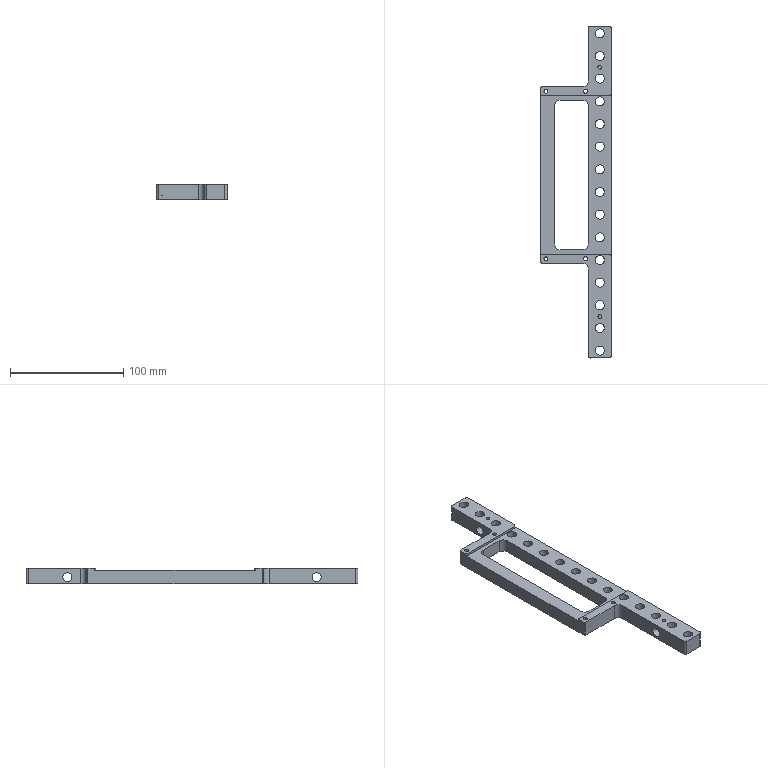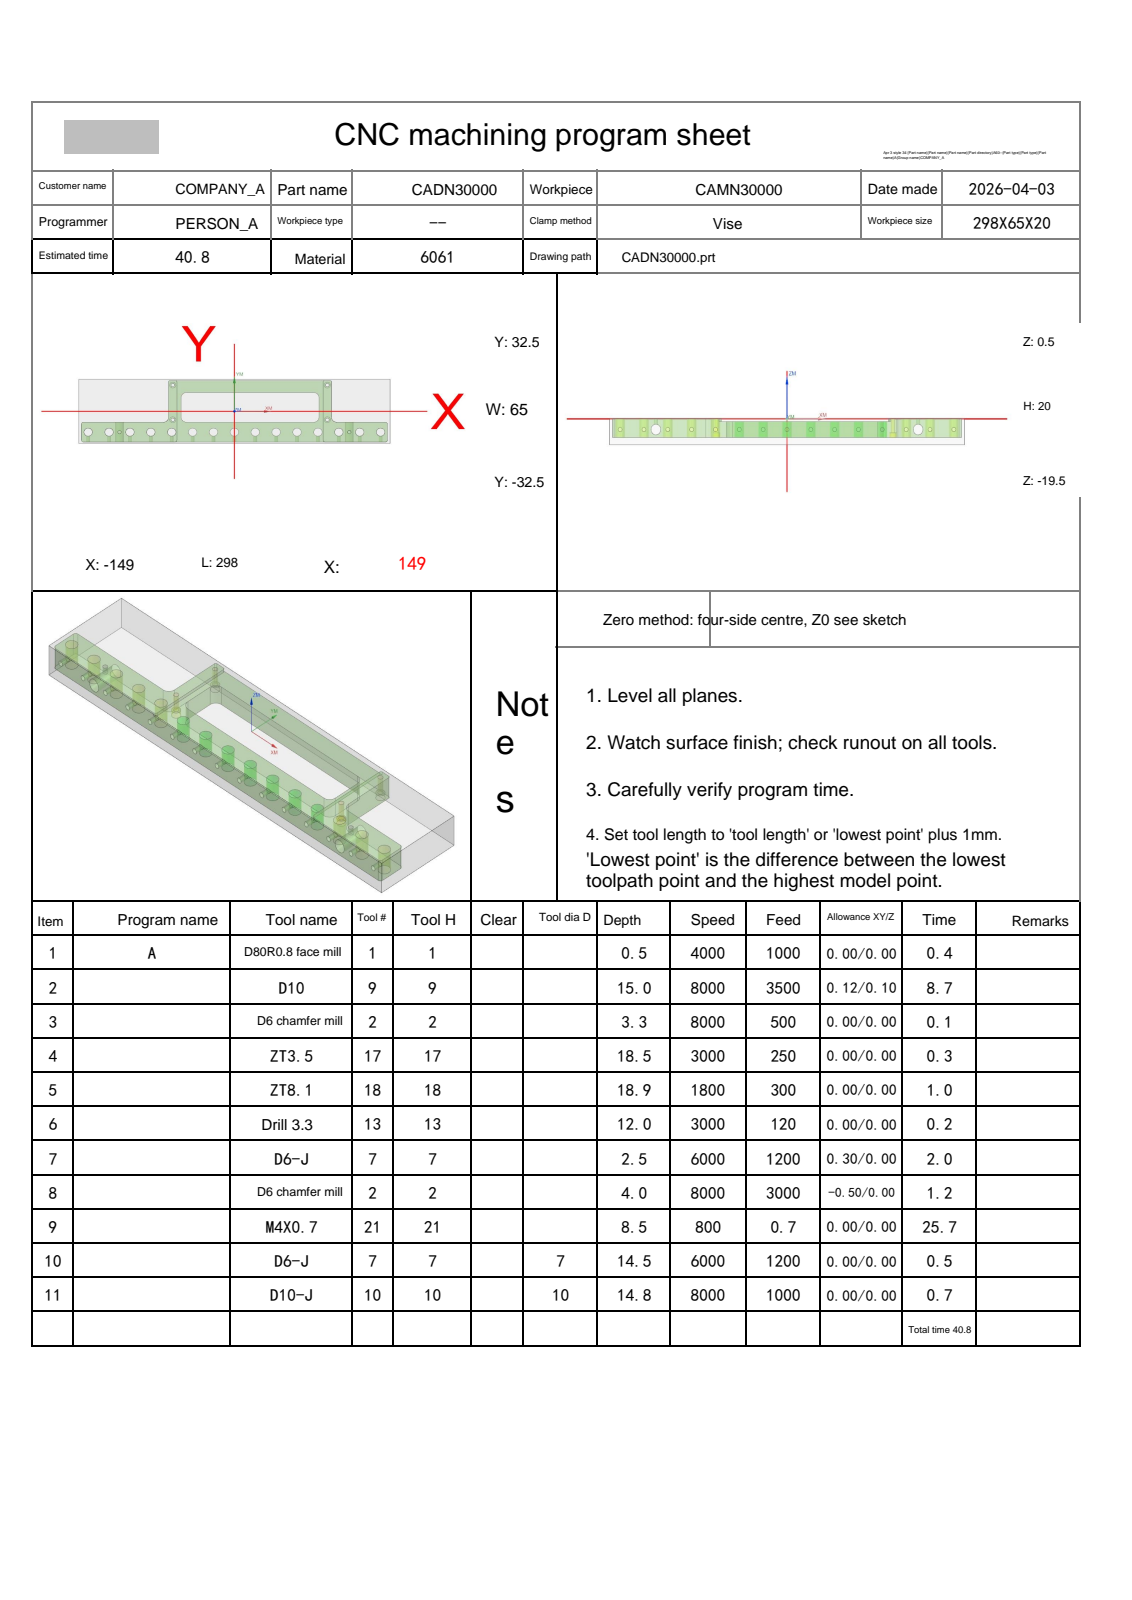NC program | NX | posted by the shop | part box 62 x 293 x 14 mm
Lines 5279 to 5964 of 5964:
N3 T02 M06
(D6 chamfer mill  D=6. R=0. H=02 ce=0.00 di=0.10)
G00 G90 G54 X-140. Y-21. M03 S8000
G43 H02 Z20.
M08
G98 G81 X-140. Y-21. Z-.8 R1. F500.
X-120.
X-110.
X-100.
X-80.
X-60.
X-59. Y-8.5
Y26.5
X-40. Y-21. Z-2.8 R-1.
X-20.
X0.0
X20.
X40.
X60.
X80.
X89. Y-8.5 Z-.8 R1.
Y26.5
X100. Y-21.
X110.
X120.
X140.
G80
G00 Z20.
G91 G28 Z0.0
M05
M09
G91 G28 Z0.0
M01
N4 T17 M06
(ZT3.5 D=3.5 DR_a=118 H=17)
G00 G90 G54 X-59. Y26.5 M03 S3000
G43 H17 Z20.
M08
G98 G83 X-59. Y26.5 Z-18. R1. F250. Q3.
Y-8.5
X89.
Y26.5
G80
G00 Z20.
G91 G28 Z0.0
M05
M09
G91 G28 Z0.0
M01
N5 T18 M06
(ZT8.1 D=8.1 DR_a=118 H=18)
G00 G90 G54 X140. Y-21. M03 S1800
G43 H18 Z20.
M08
G98 G83 X140. Y-21. Z-18.433 R1. F300. Q3.
X120.
X100.
G98 G83 X80. Y-21. Z-18.433 R-1. Q3.
X60.
X40.
X20.
X0.0
X-20.
X-40.
G98 G83 X-60. Y-21. Z-18.433 R1. Q3.
X-80.
X-100.
X-120.
X-140.
G80
G00 Z20.
G91 G28 Z0.0
M05
M09
G91 G28 Z0.0
M01
N6 T13 M06
(drill 3.3 D=3.3 DR_a=118 H=13)
G00 G90 G54 X110. Y-21. M03 S3000
G43 H13 Z20.
M08
G98 G83 X110. Y-21. Z-11.5 R1. F120. Q2.
X-110.
G80
G00 Z20.
G91 G28 Z0.0
M05
M09
G91 G28 Z0.0
M01
N7 T07 M06
(D6-J  D=6. R=0. H=07 ce=0.30 di=0.00)
G00 G90 G54 X14.056 Y-37. M03 S6000
G43 H07 Z20.
M08
Z-1.5
G01 Z-2. F1200.
X14.253 Y-31.6
G03 X14.3 Y-29. I-71.253 J2.6
G01 Y30.
G03 X14.282 Y31.6 I-70.3 J0.0
G01 X14.159 Y37.
Z-1.5
G00 Z20.
X15.841
Z-1.5
G01 Z-2.
X15.718 Y31.6
G03 X15.7 Y30. I70.282 J-1.6
G01 Y-29.
G03 X15.747 Y-31.6 I71.3 J0.0
G01 X15.944 Y-37.
Z-1.5
G00 Z20.
X11.045
Z-1.5
G01 Z-2.
X11.25 Y-31.6
G03 X11.3 Y-29. I-68.25 J2.6
G01 Y30.
G03 X11.281 Y31.6 I-67.3 J0.0
G01 X7.08
G02 X7.1 Y30. I-63.08 J-1.6
G01 Y-29.
G02 X7.047 Y-31.6 I-64.1 J0.0
G01 X2.844
G03 X2.9 Y-29. I-59.844 J2.6
G01 Y30.
G03 X2.878 Y31.6 I-58.9 J0.0
G01 X-1.323
G02 X-1.3 Y30. I-54.677 J-1.6
G01 Y-29.
G02 X-1.361 Y-31.6 I-55.7 J0.0
G01 X-5.566
G03 X-5.5 Y-29. I-51.434 J2.6
G01 Y30.
G03 X-5.525 Y31.6 I-50.5 J0.0
G01 X-9.728
G02 X-9.7 Y30. I-46.272 J-1.6
G01 Y-29.
G02 X-9.772 Y-31.6 I-47.3 J0.0
G01 X-13.978
G03 X-13.9 Y-29. I-43.022 J2.6
G01 Y30.
G03 X-13.93 Y31.6 I-42.1 J0.0
G01 X-18.134
G02 X-18.1 Y30. I-37.866 J-1.6
G01 Y-29.
G02 X-18.187 Y-31.6 I-38.9 J0.0
G01 X-22.398
G03 X-22.3 Y-29. I-34.602 J2.6
G01 Y30.
G03 X-22.338 Y31.6 I-33.7 J0.0
G01 X-26.543
G02 X-26.5 Y30. I-29.457 J-1.6
G01 Y-29.
G02 X-26.611 Y-31.6 I-30.5 J0.0
G01 X-30.829
G03 X-30.7 Y-29. I-26.171 J2.6
G01 Y30.
G03 X-30.751 Y31.6 I-25.3 J0.0
G01 X-34.961
G02 X-34.9 Y30. I-21.039 J-1.6
G01 Y-29.
G02 X-35.053 Y-31.6 I-22.1 J0.0
G01 X-39.29
G03 X-39.1 Y-29. I-17.71 J2.6
G01 Y30.
G03 X-39.176 Y31.6 I-16.9 J0.0
G01 X-43.401
G02 X-43.3 Y30. I-12.599 J-1.6
G01 Y-29.
G02 X-43.549 Y-31.6 I-13.7 J0.0
G01 X-47.863
G03 X-47.5 Y-29. I-9.137 J2.6
G01 Y30.
G03 X-47.652 Y31.6 I-8.5 J0.0
G01 X-52.009
G02 X-51.7 Y30. I-3.991 J-1.6
G01 Y-29.
G02 X-52.382 Y-31.6 I-5.3 J0.0
G01 X-55.515 Y-37.166
Z-1.5
G00 Z20.
X18.847 Y37.
Z-1.5
G01 Z-2.
X18.719 Y31.6
G03 X18.7 Y30. I67.281 J-1.6
G01 Y-29.
G03 X18.75 Y-31.6 I68.3 J0.0
G01 X22.953
G02 X22.9 Y-29. I64.047 J2.6
G01 Y30.
G02 X22.92 Y31.6 I63.1 J0.0
G01 X27.122
G03 X27.1 Y30. I58.878 J-1.6
G01 Y-29.
G03 X27.156 Y-31.6 I59.9 J0.0
G01 X31.361
G02 X31.3 Y-29. I55.639 J2.6
G01 Y30.
G02 X31.323 Y31.6 I54.7 J0.0
G01 X35.525
G03 X35.5 Y30. I50.475 J-1.6
G01 Y-29.
G03 X35.566 Y-31.6 I51.5 J0.0
G01 X39.772
G02 X39.7 Y-29. I47.228 J2.6
G01 Y30.
G02 X39.728 Y31.6 I46.3 J0.0
G01 X43.93
G03 X43.9 Y30. I42.07 J-1.6
G01 Y-29.
G03 X43.978 Y-31.6 I43.1 J0.0
G01 X48.187
G02 X48.1 Y-29. I38.813 J2.6
G01 Y30.
G02 X48.134 Y31.6 I37.9 J0.0
G01 X52.338
G03 X52.3 Y30. I33.662 J-1.6
G01 Y-29.
G03 X52.398 Y-31.6 I34.7 J0.0
G01 X56.611
G02 X56.5 Y-29. I30.389 J2.6
G01 Y30.
G02 X56.543 Y31.6 I29.5 J0.0
G01 X60.751
G03 X60.7 Y30. I25.249 J-1.6
G01 Y-29.
G03 X60.829 Y-31.6 I26.3 J0.0
G01 X65.053
G02 X64.9 Y-29. I21.947 J2.6
G01 Y30.
G02 X64.961 Y31.6 I21.1 J0.0
G01 X69.176
G03 X69.1 Y30. I16.824 J-1.6
G01 Y-29.
G03 X69.29 Y-31.6 I17.9 J0.0
G01 X73.549
G02 X73.3 Y-29. I13.451 J2.6
G01 Y30.
G02 X73.401 Y31.6 I12.7 J0.0
G01 X77.652
G03 X77.5 Y30. I8.348 J-1.6
G01 Y-29.
G03 X77.863 Y-31.6 I9.5 J0.0
G01 X82.382
G02 X81.7 Y-29. I4.618 J2.6
G01 Y30.
G02 X82.009 Y31.6 I4.3 J0.0
G01 X84.204 Y37.076
Z-1.5
G00 Z20.
G91 G28 Z0.0
M05
M09
G91 G28 Z0.0
M01
N8 T02 M06
(D6 chamfer mill  D=6. R=0. H=02 ce=0.00 di=0.00)
G00 G90 G54 X83.172 Y.25 M03 S8000
G43 H02 Z20.
M08
Z2.399
G01 Z-1.5 F3000.
G03 X83.472 Y.17 I.3 J.52
X83.992 Y.47 I0.0 J.6
G01 X84. Y.5
Y30.
G02 X86. Y32. I2. J0.0
G01 X92.
G02 X94. Y30. I0.0 J-2.
G01 Y-5.9
G03 X98.1 Y-10. I4.1 J0.0
G01 X144.5
G02 X147.5 Y-13. I0.0 J-3.
G01 Y-29.
G02 X144.5 Y-32. I-3. J0.0
G01 X87.
G02 X84. Y-29. I0.0 J3.
G01 Y.5
X83.992 Y.53
G03 X83.472 Y.83 I-.52 J-.3
X83.172 Y.75 I0.0 J-.6
G01 Z2.399
G00 Z20.
X-100.5 Y-32.828
Z2.399
G01 Z-1.5
G03 X-100.42 Y-32.528 I-.52 J.3
X-100.72 Y-32.008 I-.6 J0.0
G01 X-100.75 Y-32.
X-144.5
G02 X-147.5 Y-29. I0.0 J3.
G01 Y-13.
G02 X-144.5 Y-10. I3. J0.0
G01 X-68.1
G03 X-64. Y-5.9 I0.0 J4.1
G01 Y30.
G02 X-62. Y32. I2. J0.0
G01 X-56.
G02 X-54. Y30. I0.0 J-2.
G01 Y-29.
G02 X-57. Y-32. I-3. J0.0
G01 X-100.75
X-100.78 Y-32.008
G03 X-101.08 Y-32.528 I.3 J-.52
X-101. Y-32.828 I.6 J0.0
G01 Z2.399
G00 Z20.
X-52.193 Y32.828
Z2.055
G01 Z-3.5
G03 X-52.274 Y32.528 I.52 J-.3
X-51.974 Y32.008 I.6 J0.0
G01 X-51.944 Y32.
X81.944
X81.974 Y32.008
G03 X82.274 Y32.528 I-.3 J.52
X82.193 Y32.828 I-.6 J0.0
G01 Z2.055
G00 Z20.
X82.609 Y-32.828
Z2.055
G01 Z-3.5
G03 X82.689 Y-32.528 I-.52 J.3
X82.389 Y-32.008 I-.6 J0.0
G01 X82.359 Y-32.
X-52.359
X-52.389 Y-32.008
G03 X-52.689 Y-32.528 I.3 J-.52
X-52.609 Y-32.828 I.6 J0.0
G01 Z2.055
G00 Z20.
X14.75 Y-9.172
Z.399
G01 Z-3.5
G03 X14.67 Y-9.472 I.52 J-.3
X14.97 Y-9.992 I.6 J0.0
G01 X15. Y-10.
X75.9
G03 X80. Y-5.9 I0.0 J4.1
G01 Y13.9
G03 X75.9 Y18. I-4.1 J0.0
G01 X-45.9
G03 X-50. Y13.9 I0.0 J-4.1
G01 Y-5.9
G03 X-45.9 Y-10. I4.1 J0.0
G01 X15.
X15.03 Y-9.992
G03 X15.33 Y-9.472 I-.3 J.52
X15.25 Y-9.172 I-.6 J0.0
G01 Z.399
G00 Z20.
G00 G90 X110. Y-21. M03 S8000
Z20.
G98 G81 X110. Y-21. Z-2.2 R3. F500.
X-110.
G80
G00 Z20.
G00 G90 X-59. Y26.5 M03 S8000
Z20.
G98 G81 X-59. Y26.5 Z-2.05 R3. F500.
Y-8.5
X89.
Y26.5
G80
G00 Z20.
G00 G90 X-137.492 Y-20.54 M03 S8000
Z20.
Z-.5
G01 Z-1. F800.
X-137. Y-20.45
G03 X-140. Y-17.45 I-3. J0.0
X-143.55 Y-21. I0.0 J-3.55
X-140. Y-24.55 I3.55 J0.0
X-136.45 Y-21. I0.0 J3.55
X-140. Y-17.45 I-3.55 J0.0
X-143. Y-20.45 I0.0 J-3.
G01 X-142.508 Y-20.54
Z-.5
G00 Z20.
X-117.492
Z-.5
G01 Z-1.
X-117. Y-20.45
G03 X-120. Y-17.45 I-3. J0.0
X-123.55 Y-21. I0.0 J-3.55
X-120. Y-24.55 I3.55 J0.0
X-116.45 Y-21. I0.0 J3.55
X-120. Y-17.45 I-3.55 J0.0
X-123. Y-20.45 I0.0 J-3.
G01 X-122.508 Y-20.54
Z-.5
G00 Z20.
X-97.492
Z-.5
G01 Z-1.
X-97. Y-20.45
G03 X-100. Y-17.45 I-3. J0.0
X-103.55 Y-21. I0.0 J-3.55
X-100. Y-24.55 I3.55 J0.0
X-96.45 Y-21. I0.0 J3.55
X-100. Y-17.45 I-3.55 J0.0
X-103. Y-20.45 I0.0 J-3.
G01 X-102.508 Y-20.54
Z-.5
G00 Z20.
X-77.492
Z-.5
G01 Z-1.
X-77. Y-20.45
G03 X-80. Y-17.45 I-3. J0.0
X-83.55 Y-21. I0.0 J-3.55
X-80. Y-24.55 I3.55 J0.0
X-76.45 Y-21. I0.0 J3.55
X-80. Y-17.45 I-3.55 J0.0
X-83. Y-20.45 I0.0 J-3.
G01 X-82.508 Y-20.54
Z-.5
G00 Z20.
X-57.492
Z-.5
G01 Z-1.
X-57. Y-20.45
G03 X-60. Y-17.45 I-3. J0.0
X-63.55 Y-21. I0.0 J-3.55
X-60. Y-24.55 I3.55 J0.0
X-56.45 Y-21. I0.0 J3.55
X-60. Y-17.45 I-3.55 J0.0
X-63. Y-20.45 I0.0 J-3.
G01 X-62.508 Y-20.54
Z-.5
G00 Z20.
X-39.45 Y-20.982
Z-.5
G01 Z-1.
X-38.5 Y-20.95
G03 X-40. Y-19.45 I-1.5 J0.0
X-41.55 Y-21. I0.0 J-1.55
X-40. Y-22.55 I1.55 J0.0
X-38.45 Y-21. I0.0 J1.55
X-40. Y-19.45 I-1.55 J0.0
X-41.5 Y-20.95 I0.0 J-1.5
G01 X-40.55 Y-20.982
Z-.5
G00 Z20.
X-19.45
Z-.5
G01 Z-1.
X-18.5 Y-20.95
G03 X-20. Y-19.45 I-1.5 J0.0
X-21.55 Y-21. I0.0 J-1.55
X-20. Y-22.55 I1.55 J0.0
X-18.45 Y-21. I0.0 J1.55
X-20. Y-19.45 I-1.55 J0.0
X-21.5 Y-20.95 I0.0 J-1.5
G01 X-20.55 Y-20.982
Z-.5
G00 Z20.
X.55
Z-.5
G01 Z-1.
X1.5 Y-20.95
G03 X0.0 Y-19.45 I-1.5 J0.0
X-1.55 Y-21. I0.0 J-1.55
X0.0 Y-22.55 I1.55 J0.0
X1.55 Y-21. I0.0 J1.55
X0.0 Y-19.45 I-1.55 J0.0
X-1.5 Y-20.95 I0.0 J-1.5
G01 X-.55 Y-20.982
Z-.5
G00 Z20.
X20.55
Z-.5
G01 Z-1.
X21.5 Y-20.95
G03 X20. Y-19.45 I-1.5 J0.0
X18.45 Y-21. I0.0 J-1.55
X20. Y-22.55 I1.55 J0.0
X21.55 Y-21. I0.0 J1.55
X20. Y-19.45 I-1.55 J0.0
X18.5 Y-20.95 I0.0 J-1.5
G01 X19.45 Y-20.982
Z-.5
G00 Z20.
X40.55
Z-.5
G01 Z-1.
X41.5 Y-20.95
G03 X40. Y-19.45 I-1.5 J0.0
X38.45 Y-21. I0.0 J-1.55
X40. Y-22.55 I1.55 J0.0
X41.55 Y-21. I0.0 J1.55
X40. Y-19.45 I-1.55 J0.0
X38.5 Y-20.95 I0.0 J-1.5
G01 X39.45 Y-20.982
Z-.5
G00 Z20.
X60.55
Z-.5
G01 Z-1.
X61.5 Y-20.95
G03 X60. Y-19.45 I-1.5 J0.0
X58.45 Y-21. I0.0 J-1.55
X60. Y-22.55 I1.55 J0.0
X61.55 Y-21. I0.0 J1.55
X60. Y-19.45 I-1.55 J0.0
X58.5 Y-20.95 I0.0 J-1.5
G01 X59.45 Y-20.982
Z-.5
G00 Z20.
X80.55
Z-.5
G01 Z-1.
X81.5 Y-20.95
G03 X80. Y-19.45 I-1.5 J0.0
X78.45 Y-21. I0.0 J-1.55
X80. Y-22.55 I1.55 J0.0
X81.55 Y-21. I0.0 J1.55
X80. Y-19.45 I-1.55 J0.0
X78.5 Y-20.95 I0.0 J-1.5
G01 X79.45 Y-20.982
Z-.5
G00 Z20.
X102.508 Y-20.54
Z-.5
G01 Z-1.
X103. Y-20.45
G03 X100. Y-17.45 I-3. J0.0
X96.45 Y-21. I0.0 J-3.55
X100. Y-24.55 I3.55 J0.0
X103.55 Y-21. I0.0 J3.55
X100. Y-17.45 I-3.55 J0.0
X97. Y-20.45 I0.0 J-3.
G01 X97.492 Y-20.54
Z-.5
G00 Z20.
X122.508
Z-.5
G01 Z-1.
X123. Y-20.45
G03 X120. Y-17.45 I-3. J0.0
X116.45 Y-21. I0.0 J-3.55
X120. Y-24.55 I3.55 J0.0
X123.55 Y-21. I0.0 J3.55
X120. Y-17.45 I-3.55 J0.0
X117. Y-20.45 I0.0 J-3.
G01 X117.492 Y-20.54
Z-.5
G00 Z20.
X142.508
Z-.5
G01 Z-1.
X143. Y-20.45
G03 X140. Y-17.45 I-3. J0.0
X136.45 Y-21. I0.0 J-3.55
X140. Y-24.55 I3.55 J0.0
X143.55 Y-21. I0.0 J3.55
X140. Y-17.45 I-3.55 J0.0
X137. Y-20.45 I0.0 J-3.
G01 X137.492 Y-20.54
Z-.5
G00 Z20.
G91 G28 Z0.0
M05
M09
G91 G28 Z0.0
M01
N9 T21 M06
(M4X0.7 D=3.3 DR_a=180 H=21)
G00 G90 G54 X110. Y-21. M03 S800
G43 H21 Z20.
M08
G95
G98 G84 X110. Y-21. Z-8. R1. F.7 Q3.
X-110.
G80
G94
G00 Z20.
G91 G28 Z0.0
M05
M09
G91 G28 Z0.0
M01
N10 T07 M06
(D6-J  D=6. R=0. H=07 ce=0.00 di=0.01)
G00 G90 G54 X90.7 Y-35.1 M03 S6000
G43 H07 Z20.
M08
Z-1.495
G01 Z-1.995 F1200.
G41 D07
Y-35.
G03 X89.7 Y-34. I-1. J0.0
G01 X87.
G02 X82. Y-29. I0.0 J5.
G01 Y30.
G02 X86. Y34. I4. J0.0
G01 X88.7
G03 X89.7 Y35. I0.0 J1.
G01 G40 Y35.1
Z-1.495
G00 Z20.
X-59.7
Z-1.495
G01 Z-1.995
G41 D07
Y35.
G03 X-58.7 Y34. I1. J0.0
G01 X-56.
G02 X-52. Y30. I0.0 J-4.
G01 Y-29.
G02 X-57. Y-34. I-5. J0.0
G01 X-59.7
G03 X-60.7 Y-35. I0.0 J-1.
G01 G40 Y-35.1
Z-1.495
G00 Z20.
G00 G90 X76.9 Y14.258 M03 S6000
Z20.
Z-13.5
G01 Z-14. F1000.
G41 D07
Y15.
G03 X75.9 Y16. I-1. J0.0
G01 X-45.9
G03 X-48. Y13.9 I0.0 J-2.1
G01 Y-5.9
G03 X-45.9 Y-8. I2.1 J0.0
G01 X75.9
G03 X78. Y-5.9 I0.0 J2.1
G01 Y13.9
G03 X75.9 Y16. I-2.1 J0.0
G01 X75.4
G03 X74.4 Y15. I0.0 J-1.
G01 G40 Y14.9
Z-13.5
G00 Z20.
G91 G28 Z0.0
M05
M09
G91 G28 Z0.0
M01
N11 T10 M06
(D10-J  D=10. R=0. H=10 ce=0.00 di=0.00)
G00 G90 G54 X145.511 Y-37.137 M03 S8000
G43 H10 Z20.
M08
Z-13.8
G01 Z-14.3 F1000.
G41 D10
X145.498 Y-36.938
G03 X144.5 Y-36. I-.998 J-.063
G01 X-144.5
G02 X-151.5 Y-29. I0.0 J7.
G01 Y-13.
G02 X-144.5 Y-6. I7. J0.0
G01 X-68.1
X-68.045 Y-5.995
X-68.005 Y-5.955
X-68. Y-5.9
Y30.
G02 X-62. Y36. I6. J0.0
G01 X92.
G02 X98. Y30. I0.0 J-6.
G01 Y-5.9
X98.005 Y-5.955
X98.045 Y-5.995
X98.1 Y-6.
X144.5
G02 X151.5 Y-13. I0.0 J-7.
G01 Y-29.
G02 X144.5 Y-36. I-7. J0.0
G01 X144.
G03 X143. Y-37. I0.0 J-1.
G01 G40 Y-37.2
Z-13.8
G00 Z20.
M05
M09
G91 G28 Z0.0
G91 G28 Y0.0
M30
%